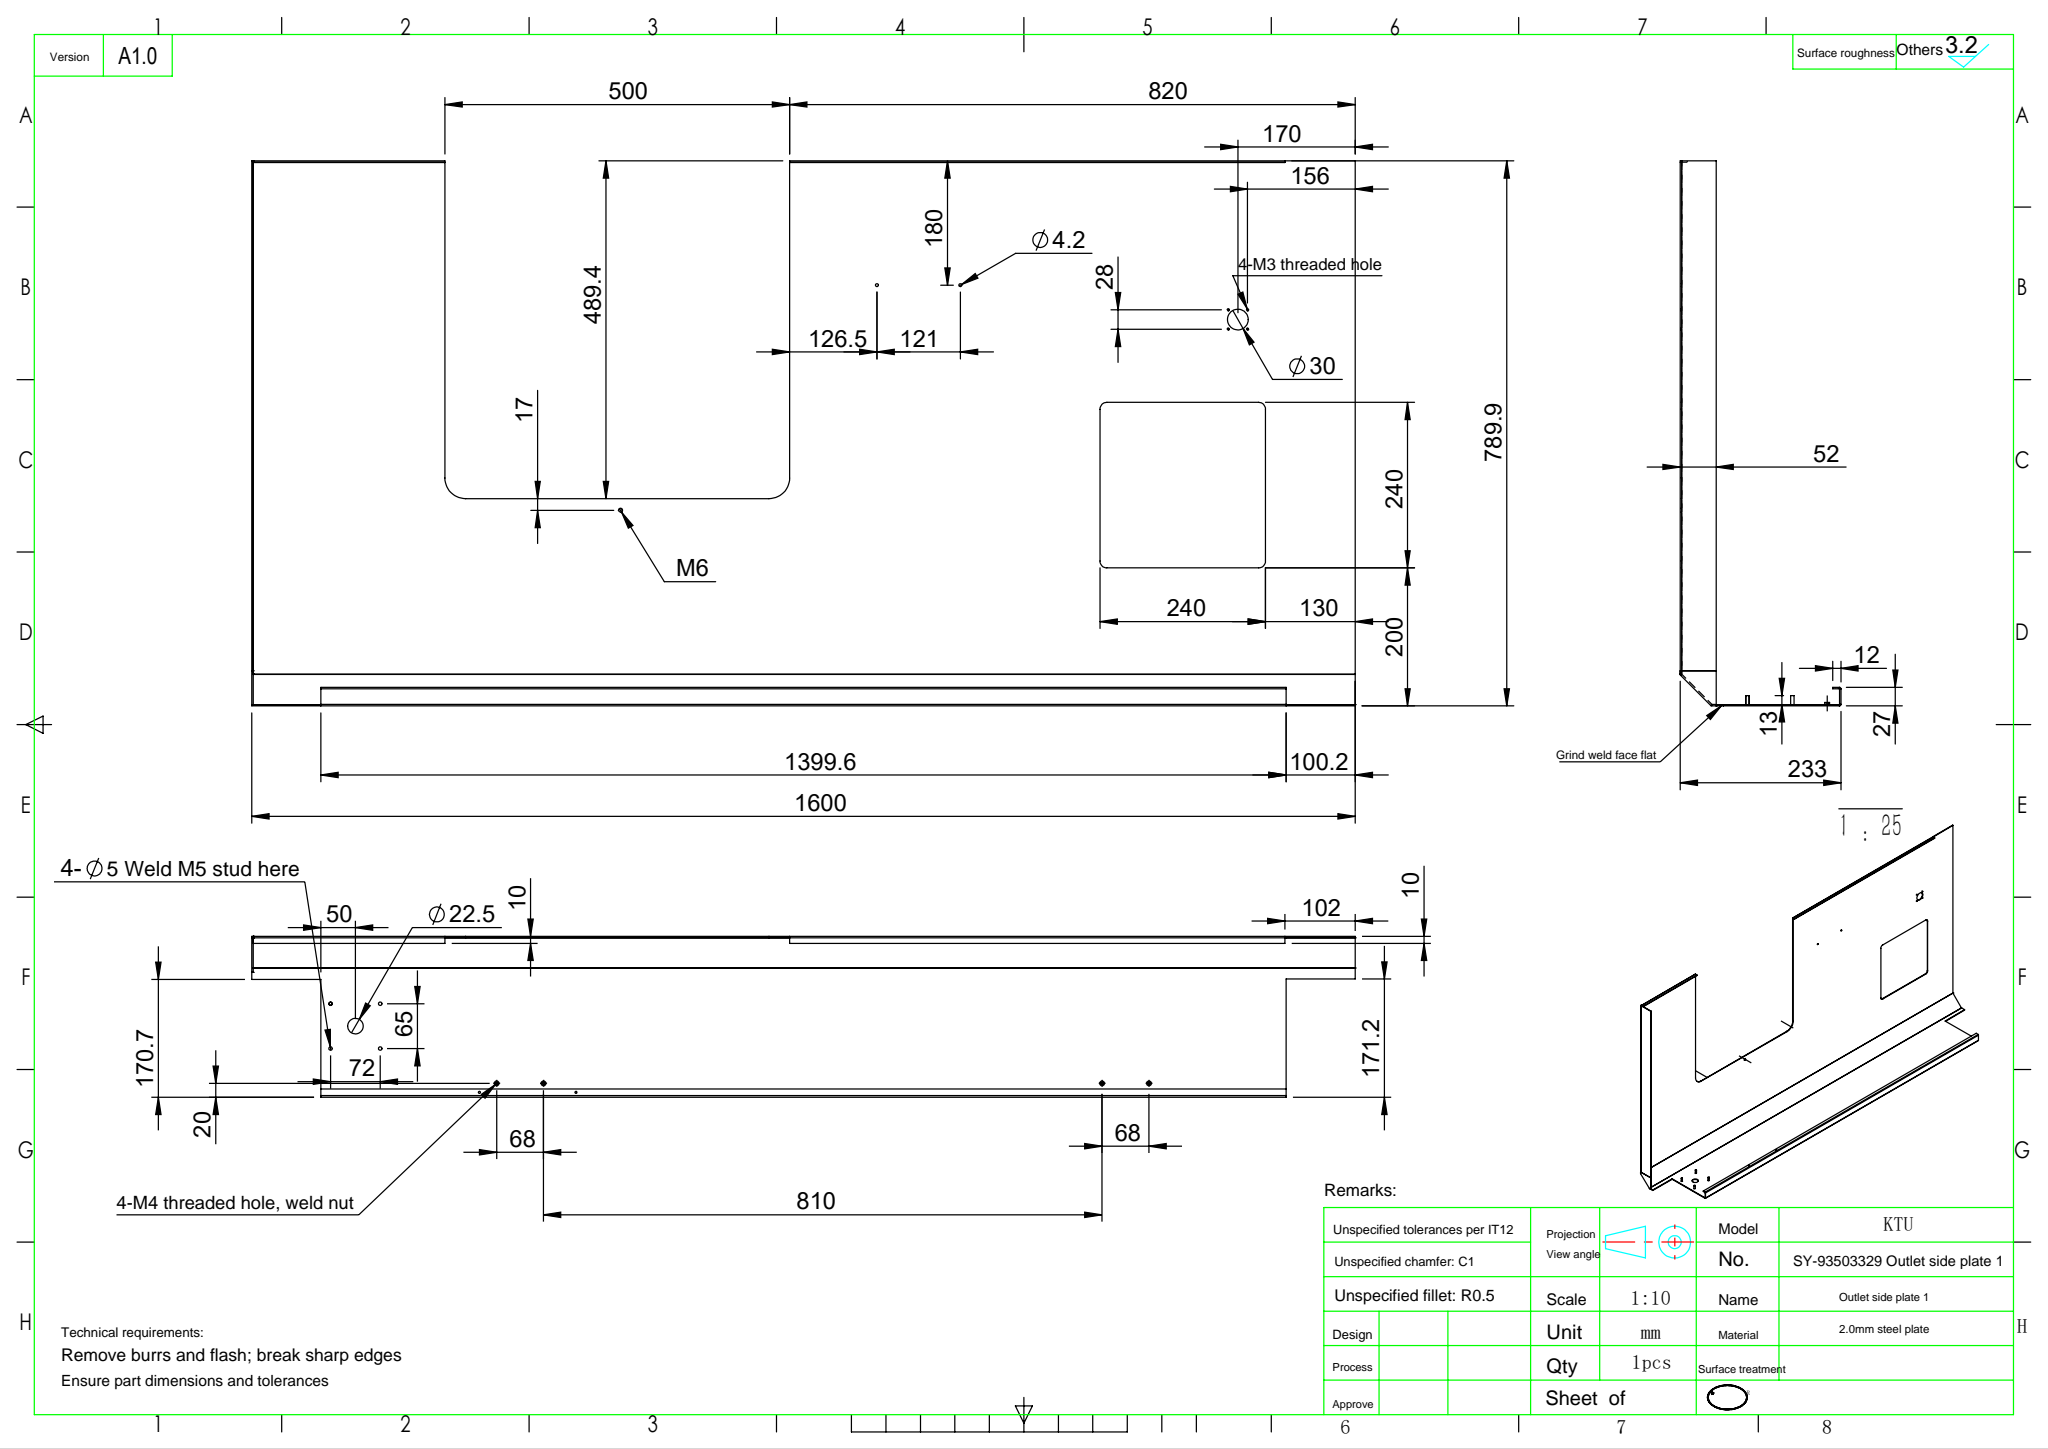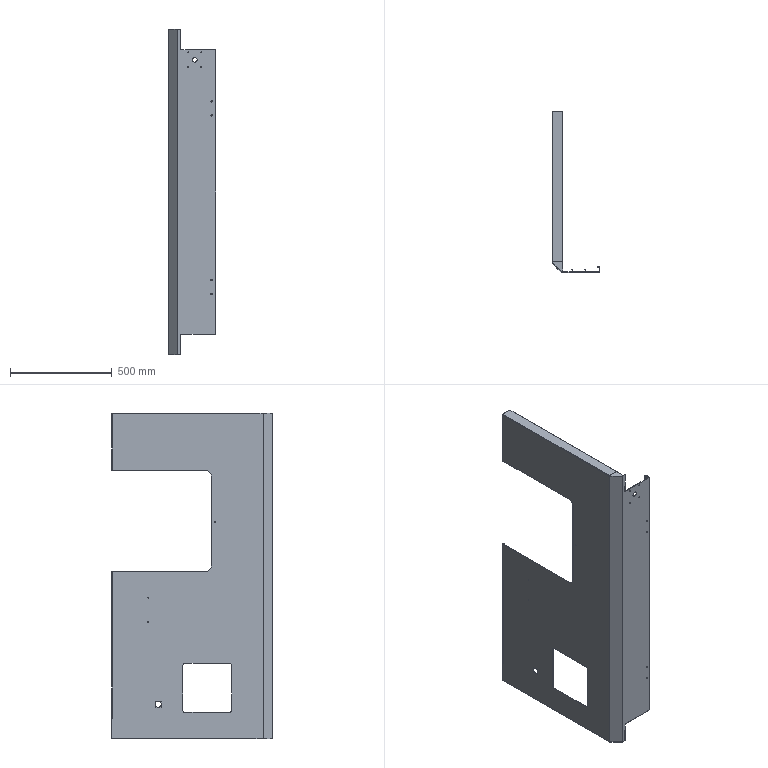Part | SolidWorks | features ICE 10, Cut 4, EdgeFlange 4, HoleWzd 4, 3DProfileFeature 2, FlatPattern 2, SMBaseFlange 2, SheetMetal 2, DelFace 1 | 6 solids | 165 faces | box 233 x 789.9 x 1600 mm | volume 2696095 mm3 | plane 88 | cylinder 77 | commonest cylinder face diameters 5 x16 2.5 x8 3.3 x8 4.4 x8 7 x8 0.4 x7